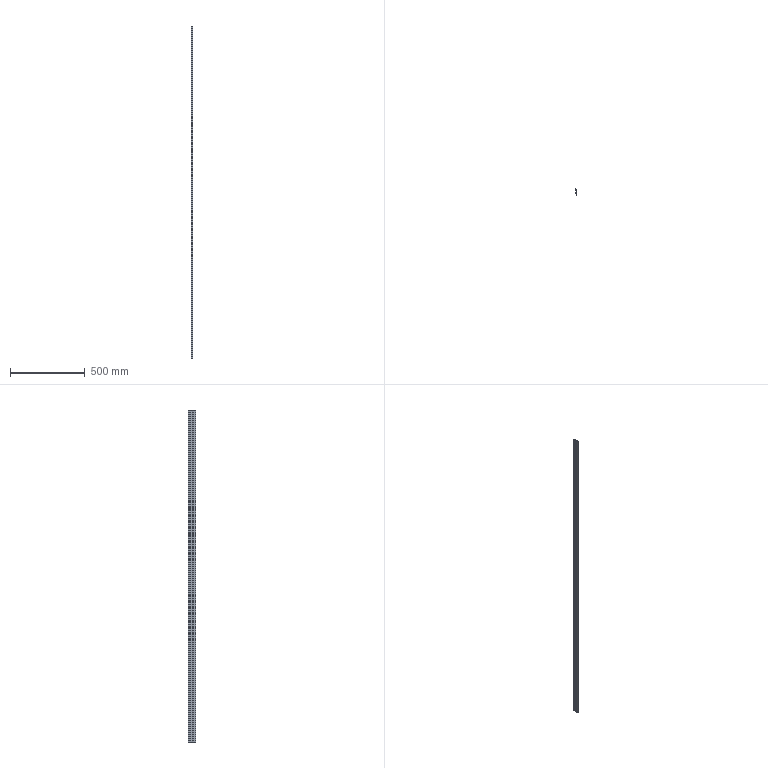Part | SolidWorks | features Extrusion 1 | 1 solid | 33 faces | box 9.4 x 46.998 x 2216 mm | volume 250321 mm3 | plane 22 | cylinder 11 | commonest cylinder face diameters 0.24 x2 0.4 x2 0.8 x2 1.2 x2 6 x2 1 x1
STEP:
#1=CARTESIAN_POINT('',(-2.9,32.45,-1108.));
#2=VERTEX_POINT('',#1);
#3=CARTESIAN_POINT('',(-2.7,32.25,-1108.));
#4=VERTEX_POINT('',#3);
#5=CARTESIAN_POINT('',(-2.7,32.45,-1108.));
#6=DIRECTION('',(0.,0.,1.));
#7=DIRECTION('',(1.,0.,0.));
#8=AXIS2_PLACEMENT_3D('',#5,#6,#7);
#9=CIRCLE('',#8,0.2);
#10=EDGE_CURVE('',#2,#4,#9,.T.);
#11=ORIENTED_EDGE('',*,*,#10,.T.);
#12=CARTESIAN_POINT('',(-2.7,32.25,1108.));
#13=VERTEX_POINT('',#12);
#14=CARTESIAN_POINT('',(-2.7,32.25,1108.));
#15=DIRECTION('',(0.,0.,-1.));
#16=VECTOR('',#15,1000.);
#17=LINE('',#14,#16);
#18=EDGE_CURVE('',#13,#4,#17,.T.);
#19=ORIENTED_EDGE('',*,*,#18,.F.);
#20=CARTESIAN_POINT('',(-2.9,32.45,1108.));
#21=VERTEX_POINT('',#20);
#22=CARTESIAN_POINT('',(-2.7,32.45,1108.));
#23=DIRECTION('',(0.,0.,1.));
#24=DIRECTION('',(1.,0.,0.));
#25=AXIS2_PLACEMENT_3D('',#22,#23,#24);
#26=CIRCLE('',#25,0.2);
#27=EDGE_CURVE('',#21,#13,#26,.T.);
#28=ORIENTED_EDGE('',*,*,#27,.F.);
#29=CARTESIAN_POINT('',(-2.9,32.45,1108.));
#30=DIRECTION('',(0.,0.,-1.));
#31=VECTOR('',#30,1000.);
#32=LINE('',#29,#31);
#33=EDGE_CURVE('',#21,#2,#32,.T.);
#34=ORIENTED_EDGE('',*,*,#33,.T.);
#35=EDGE_LOOP('',(#11,#19,#28,#34));
#36=FACE_OUTER_BOUND('',#35,.T.);
#37=CARTESIAN_POINT('',(-2.7,32.45,1108.));
#38=DIRECTION('',(0.,0.,-1.));
#39=DIRECTION('',(-1.,0.,0.));
#40=AXIS2_PLACEMENT_3D('',#37,#38,#39);
#41=CYLINDRICAL_SURFACE('',#40,0.2);
#42=ADVANCED_FACE('',(#36),#41,.T.);
#43=CARTESIAN_POINT('',(-2.5,32.25,-1108.));
#44=VERTEX_POINT('',#43);
#45=CARTESIAN_POINT('',(-2.7,32.25,-1108.));
#46=DIRECTION('',(1.,0.,0.));
#47=VECTOR('',#46,1000.);
#48=LINE('',#45,#47);
#49=EDGE_CURVE('',#4,#44,#48,.T.);
#50=ORIENTED_EDGE('',*,*,#49,.T.);
#51=CARTESIAN_POINT('',(-2.5,32.25,1108.));
#52=VERTEX_POINT('',#51);
#53=CARTESIAN_POINT('',(-2.5,32.25,1108.));
#54=DIRECTION('',(0.,0.,-1.));
#55=VECTOR('',#54,1000.);
#56=LINE('',#53,#55);
#57=EDGE_CURVE('',#52,#44,#56,.T.);
#58=ORIENTED_EDGE('',*,*,#57,.F.);
#59=CARTESIAN_POINT('',(-2.7,32.25,1108.));
#60=DIRECTION('',(1.,0.,0.));
#61=VECTOR('',#60,1000.);
#62=LINE('',#59,#61);
#63=EDGE_CURVE('',#13,#52,#62,.T.);
#64=ORIENTED_EDGE('',*,*,#63,.F.);
#65=ORIENTED_EDGE('',*,*,#18,.T.);
#66=EDGE_LOOP('',(#50,#58,#64,#65));
#67=FACE_OUTER_BOUND('',#66,.T.);
#68=CARTESIAN_POINT('',(-2.7,32.25,1108.));
#69=DIRECTION('',(0.,1.,0.));
#70=DIRECTION('',(0.,0.,1.));
#71=AXIS2_PLACEMENT_3D('',#68,#69,#70);
#72=PLANE('',#71);
#73=ADVANCED_FACE('',(#67),#72,.F.);
#74=CARTESIAN_POINT('',(-1.9,32.85,-1108.));
#75=VERTEX_POINT('',#74);
#76=CARTESIAN_POINT('',(-2.5,32.85,-1108.));
#77=DIRECTION('',(0.,0.,1.));
#78=DIRECTION('',(1.,0.,0.));
#79=AXIS2_PLACEMENT_3D('',#76,#77,#78);
#80=CIRCLE('',#79,0.6);
#81=EDGE_CURVE('',#44,#75,#80,.T.);
#82=ORIENTED_EDGE('',*,*,#81,.T.);
#83=CARTESIAN_POINT('',(-1.9,32.85,1108.));
#84=VERTEX_POINT('',#83);
#85=CARTESIAN_POINT('',(-1.9,32.85,1108.));
#86=DIRECTION('',(0.,0.,-1.));
#87=VECTOR('',#86,1000.);
#88=LINE('',#85,#87);
#89=EDGE_CURVE('',#84,#75,#88,.T.);
#90=ORIENTED_EDGE('',*,*,#89,.F.);
#91=CARTESIAN_POINT('',(-2.5,32.85,1108.));
#92=DIRECTION('',(0.,0.,1.));
#93=DIRECTION('',(1.,0.,0.));
#94=AXIS2_PLACEMENT_3D('',#91,#92,#93);
#95=CIRCLE('',#94,0.6);
#96=EDGE_CURVE('',#52,#84,#95,.T.);
#97=ORIENTED_EDGE('',*,*,#96,.F.);
#98=ORIENTED_EDGE('',*,*,#57,.T.);
#99=EDGE_LOOP('',(#82,#90,#97,#98));
#100=FACE_OUTER_BOUND('',#99,.T.);
#101=CARTESIAN_POINT('',(-2.5,32.85,1108.));
#102=DIRECTION('',(0.,0.,-1.));
#103=DIRECTION('',(-1.,0.,0.));
#104=AXIS2_PLACEMENT_3D('',#101,#102,#103);
#105=CYLINDRICAL_SURFACE('',#104,0.6);
#106=ADVANCED_FACE('',(#100),#105,.T.);
#107=CARTESIAN_POINT('',(-1.9,36.13,-1108.));
#108=VERTEX_POINT('',#107);
#109=CARTESIAN_POINT('',(-1.9,32.85,-1108.));
#110=DIRECTION('',(0.,1.,0.));
#111=VECTOR('',#110,1000.);
#112=LINE('',#109,#111);
#113=EDGE_CURVE('',#75,#108,#112,.T.);
#114=ORIENTED_EDGE('',*,*,#113,.T.);
#115=CARTESIAN_POINT('',(-1.9,36.13,1108.));
#116=VERTEX_POINT('',#115);
#117=CARTESIAN_POINT('',(-1.9,36.13,1108.));
#118=DIRECTION('',(0.,0.,-1.));
#119=VECTOR('',#118,1000.);
#120=LINE('',#117,#119);
#121=EDGE_CURVE('',#116,#108,#120,.T.);
#122=ORIENTED_EDGE('',*,*,#121,.F.);
#123=CARTESIAN_POINT('',(-1.9,32.85,1108.));
#124=DIRECTION('',(0.,1.,0.));
#125=VECTOR('',#124,1000.);
#126=LINE('',#123,#125);
#127=EDGE_CURVE('',#84,#116,#126,.T.);
#128=ORIENTED_EDGE('',*,*,#127,.F.);
#129=ORIENTED_EDGE('',*,*,#89,.T.);
#130=EDGE_LOOP('',(#114,#122,#128,#129));
#131=FACE_OUTER_BOUND('',#130,.T.);
#132=CARTESIAN_POINT('',(-1.9,32.85,1108.));
#133=DIRECTION('',(-1.,0.,0.));
#134=DIRECTION('',(0.,0.,1.));
#135=AXIS2_PLACEMENT_3D('',#132,#133,#134);
#136=PLANE('',#135);
#137=ADVANCED_FACE('',(#131),#136,.F.);
#138=CARTESIAN_POINT('',(-1.78,36.25,-1108.));
#139=VERTEX_POINT('',#138);
#140=CARTESIAN_POINT('',(-1.78,36.13,-1108.));
#141=DIRECTION('',(0.,0.,-1.));
#142=DIRECTION('',(1.,0.,0.));
#143=AXIS2_PLACEMENT_3D('',#140,#141,#142);
#144=CIRCLE('',#143,0.12);
#145=EDGE_CURVE('',#108,#139,#144,.T.);
#146=ORIENTED_EDGE('',*,*,#145,.T.);
#147=CARTESIAN_POINT('',(-1.78,36.25,1108.));
#148=VERTEX_POINT('',#147);
#149=CARTESIAN_POINT('',(-1.78,36.25,1108.));
#150=DIRECTION('',(0.,0.,-1.));
#151=VECTOR('',#150,1000.);
#152=LINE('',#149,#151);
#153=EDGE_CURVE('',#148,#139,#152,.T.);
#154=ORIENTED_EDGE('',*,*,#153,.F.);
#155=CARTESIAN_POINT('',(-1.78,36.13,1108.));
#156=DIRECTION('',(0.,0.,-1.));
#157=DIRECTION('',(1.,0.,0.));
#158=AXIS2_PLACEMENT_3D('',#155,#156,#157);
#159=CIRCLE('',#158,0.12);
#160=EDGE_CURVE('',#116,#148,#159,.T.);
#161=ORIENTED_EDGE('',*,*,#160,.F.);
#162=ORIENTED_EDGE('',*,*,#121,.T.);
#163=EDGE_LOOP('',(#146,#154,#161,#162));
#164=FACE_OUTER_BOUND('',#163,.T.);
#165=CARTESIAN_POINT('',(-1.78,36.13,1108.));
#166=DIRECTION('',(0.,0.,-1.));
#167=DIRECTION('',(-1.,0.,0.));
#168=AXIS2_PLACEMENT_3D('',#165,#166,#167);
#169=CYLINDRICAL_SURFACE('',#168,0.12);
#170=ADVANCED_FACE('',(#164),#169,.F.);
#171=CARTESIAN_POINT('',(0.,36.25,-1108.));
#172=VERTEX_POINT('',#171);
#173=CARTESIAN_POINT('',(-1.78,36.25,-1108.));
#174=DIRECTION('',(1.,0.,0.));
#175=VECTOR('',#174,1000.);
#176=LINE('',#173,#175);
#177=EDGE_CURVE('',#139,#172,#176,.T.);
#178=ORIENTED_EDGE('',*,*,#177,.T.);
#179=CARTESIAN_POINT('',(0.,36.25,1108.));
#180=VERTEX_POINT('',#179);
#181=CARTESIAN_POINT('',(0.,36.25,1108.));
#182=DIRECTION('',(0.,0.,-1.));
#183=VECTOR('',#182,1000.);
#184=LINE('',#181,#183);
#185=EDGE_CURVE('',#180,#172,#184,.T.);
#186=ORIENTED_EDGE('',*,*,#185,.F.);
#187=CARTESIAN_POINT('',(-1.78,36.25,1108.));
#188=DIRECTION('',(1.,0.,0.));
#189=VECTOR('',#188,1000.);
#190=LINE('',#187,#189);
#191=EDGE_CURVE('',#148,#180,#190,.T.);
#192=ORIENTED_EDGE('',*,*,#191,.F.);
#193=ORIENTED_EDGE('',*,*,#153,.T.);
#194=EDGE_LOOP('',(#178,#186,#192,#193));
#195=FACE_OUTER_BOUND('',#194,.T.);
#196=CARTESIAN_POINT('',(-1.78,36.25,1108.));
#197=DIRECTION('',(0.,1.,0.));
#198=DIRECTION('',(0.,0.,1.));
#199=AXIS2_PLACEMENT_3D('',#196,#197,#198);
#200=PLANE('',#199);
#201=ADVANCED_FACE('',(#195),#200,.F.);
#202=CARTESIAN_POINT('',(0.0007641,20.449,-1108.));
#203=VERTEX_POINT('',#202);
#204=CARTESIAN_POINT('',(0.,36.25,-1108.));
#205=DIRECTION('',(0.00004836,-1.,0.));
#206=VECTOR('',#205,1000.);
#207=LINE('',#204,#206);
#208=EDGE_CURVE('',#172,#203,#207,.T.);
#209=ORIENTED_EDGE('',*,*,#208,.T.);
#210=CARTESIAN_POINT('',(0.0007641,20.449,1108.));
#211=VERTEX_POINT('',#210);
#212=CARTESIAN_POINT('',(0.0007641,20.449,1108.));
#213=DIRECTION('',(0.,0.,-1.));
#214=VECTOR('',#213,1000.);
#215=LINE('',#212,#214);
#216=EDGE_CURVE('',#211,#203,#215,.T.);
#217=ORIENTED_EDGE('',*,*,#216,.F.);
#218=CARTESIAN_POINT('',(0.,36.25,1108.));
#219=DIRECTION('',(0.00004836,-1.,0.));
#220=VECTOR('',#219,1000.);
#221=LINE('',#218,#220);
#222=EDGE_CURVE('',#180,#211,#221,.T.);
#223=ORIENTED_EDGE('',*,*,#222,.F.);
#224=ORIENTED_EDGE('',*,*,#185,.T.);
#225=EDGE_LOOP('',(#209,#217,#223,#224));
#226=FACE_OUTER_BOUND('',#225,.T.);
#227=CARTESIAN_POINT('',(0.,36.25,1108.));
#228=DIRECTION('',(1.,0.00004836,0.));
#229=DIRECTION('',(-0.00004836,1.,0.));
#230=AXIS2_PLACEMENT_3D('',#227,#228,#229);
#231=PLANE('',#230);
#232=ADVANCED_FACE('',(#226),#231,.F.);
#233=CARTESIAN_POINT('',(-2.499,20.449,-1108.));
#234=VERTEX_POINT('',#233);
#235=CARTESIAN_POINT('',(0.0007641,20.449,-1108.));
#236=DIRECTION('',(-1.,0.,0.));
#237=VECTOR('',#236,1000.);
#238=LINE('',#235,#237);
#239=EDGE_CURVE('',#203,#234,#238,.T.);
#240=ORIENTED_EDGE('',*,*,#239,.T.);
#241=CARTESIAN_POINT('',(-2.499,20.449,1108.));
#242=VERTEX_POINT('',#241);
#243=CARTESIAN_POINT('',(-2.499,20.449,1108.));
#244=DIRECTION('',(0.,0.,-1.));
#245=VECTOR('',#244,1000.);
#246=LINE('',#243,#245);
#247=EDGE_CURVE('',#242,#234,#246,.T.);
#248=ORIENTED_EDGE('',*,*,#247,.F.);
#249=CARTESIAN_POINT('',(0.0007641,20.449,1108.));
#250=DIRECTION('',(-1.,0.,0.));
#251=VECTOR('',#250,1000.);
#252=LINE('',#249,#251);
#253=EDGE_CURVE('',#211,#242,#252,.T.);
#254=ORIENTED_EDGE('',*,*,#253,.F.);
#255=ORIENTED_EDGE('',*,*,#216,.T.);
#256=EDGE_LOOP('',(#240,#248,#254,#255));
#257=FACE_OUTER_BOUND('',#256,.T.);
#258=CARTESIAN_POINT('',(0.0007641,20.449,1108.));
#259=DIRECTION('',(0.,-1.,0.));
#260=DIRECTION('',(0.,0.,-1.));
#261=AXIS2_PLACEMENT_3D('',#258,#259,#260);
#262=PLANE('',#261);
#263=ADVANCED_FACE('',(#257),#262,.F.);
#264=CARTESIAN_POINT('',(-2.899,20.049,-1108.));
#265=VERTEX_POINT('',#264);
#266=CARTESIAN_POINT('',(-2.499,20.049,-1108.));
#267=DIRECTION('',(0.,0.,1.));
#268=DIRECTION('',(1.,0.,0.));
#269=AXIS2_PLACEMENT_3D('',#266,#267,#268);
#270=CIRCLE('',#269,0.4);
#271=EDGE_CURVE('',#234,#265,#270,.T.);
#272=ORIENTED_EDGE('',*,*,#271,.T.);
#273=CARTESIAN_POINT('',(-2.899,20.049,1108.));
#274=VERTEX_POINT('',#273);
#275=CARTESIAN_POINT('',(-2.899,20.049,1108.));
#276=DIRECTION('',(0.,0.,-1.));
#277=VECTOR('',#276,1000.);
#278=LINE('',#275,#277);
#279=EDGE_CURVE('',#274,#265,#278,.T.);
#280=ORIENTED_EDGE('',*,*,#279,.F.);
#281=CARTESIAN_POINT('',(-2.499,20.049,1108.));
#282=DIRECTION('',(0.,0.,1.));
#283=DIRECTION('',(1.,0.,0.));
#284=AXIS2_PLACEMENT_3D('',#281,#282,#283);
#285=CIRCLE('',#284,0.4);
#286=EDGE_CURVE('',#242,#274,#285,.T.);
#287=ORIENTED_EDGE('',*,*,#286,.F.);
#288=ORIENTED_EDGE('',*,*,#247,.T.);
#289=EDGE_LOOP('',(#272,#280,#287,#288));
#290=FACE_OUTER_BOUND('',#289,.T.);
#291=CARTESIAN_POINT('',(-2.499,20.049,1108.));
#292=DIRECTION('',(0.,0.,-1.));
#293=DIRECTION('',(-1.,0.,0.));
#294=AXIS2_PLACEMENT_3D('',#291,#292,#293);
#295=CYLINDRICAL_SURFACE('',#294,0.4);
#296=ADVANCED_FACE('',(#290),#295,.T.);
#297=CARTESIAN_POINT('',(-2.899,15.65,-1108.));
#298=VERTEX_POINT('',#297);
#299=CARTESIAN_POINT('',(-2.899,20.049,-1108.));
#300=DIRECTION('',(0.,-1.,0.));
#301=VECTOR('',#300,1000.);
#302=LINE('',#299,#301);
#303=EDGE_CURVE('',#265,#298,#302,.T.);
#304=ORIENTED_EDGE('',*,*,#303,.T.);
#305=CARTESIAN_POINT('',(-2.899,15.65,1108.));
#306=VERTEX_POINT('',#305);
#307=CARTESIAN_POINT('',(-2.899,15.65,1108.));
#308=DIRECTION('',(0.,0.,-1.));
#309=VECTOR('',#308,1000.);
#310=LINE('',#307,#309);
#311=EDGE_CURVE('',#306,#298,#310,.T.);
#312=ORIENTED_EDGE('',*,*,#311,.F.);
#313=CARTESIAN_POINT('',(-2.899,20.049,1108.));
#314=DIRECTION('',(0.,-1.,0.));
#315=VECTOR('',#314,1000.);
#316=LINE('',#313,#315);
#317=EDGE_CURVE('',#274,#306,#316,.T.);
#318=ORIENTED_EDGE('',*,*,#317,.F.);
#319=ORIENTED_EDGE('',*,*,#279,.T.);
#320=EDGE_LOOP('',(#304,#312,#318,#319));
#321=FACE_OUTER_BOUND('',#320,.T.);
#322=CARTESIAN_POINT('',(-2.899,20.049,1108.));
#323=DIRECTION('',(1.,0.,0.));
#324=DIRECTION('',(0.,0.,-1.));
#325=AXIS2_PLACEMENT_3D('',#322,#323,#324);
#326=PLANE('',#325);
#327=ADVANCED_FACE('',(#321),#326,.F.);
#328=CARTESIAN_POINT('',(-2.699,15.45,-1108.));
#329=VERTEX_POINT('',#328);
#330=CARTESIAN_POINT('',(-2.699,15.65,-1108.));
#331=DIRECTION('',(0.,0.,1.));
#332=DIRECTION('',(1.,0.,0.));
#333=AXIS2_PLACEMENT_3D('',#330,#331,#332);
#334=CIRCLE('',#333,0.2);
#335=EDGE_CURVE('',#298,#329,#334,.T.);
#336=ORIENTED_EDGE('',*,*,#335,.T.);
#337=CARTESIAN_POINT('',(-2.699,15.45,1108.));
#338=VERTEX_POINT('',#337);
#339=CARTESIAN_POINT('',(-2.699,15.45,1108.));
#340=DIRECTION('',(0.,0.,-1.));
#341=VECTOR('',#340,1000.);
#342=LINE('',#339,#341);
#343=EDGE_CURVE('',#338,#329,#342,.T.);
#344=ORIENTED_EDGE('',*,*,#343,.F.);
#345=CARTESIAN_POINT('',(-2.699,15.65,1108.));
#346=DIRECTION('',(0.,0.,1.));
#347=DIRECTION('',(1.,0.,0.));
#348=AXIS2_PLACEMENT_3D('',#345,#346,#347);
#349=CIRCLE('',#348,0.2);
#350=EDGE_CURVE('',#306,#338,#349,.T.);
#351=ORIENTED_EDGE('',*,*,#350,.F.);
#352=ORIENTED_EDGE('',*,*,#311,.T.);
#353=EDGE_LOOP('',(#336,#344,#351,#352));
#354=FACE_OUTER_BOUND('',#353,.T.);
#355=CARTESIAN_POINT('',(-2.699,15.65,1108.));
#356=DIRECTION('',(0.,0.,-1.));
#357=DIRECTION('',(-1.,0.,0.));
#358=AXIS2_PLACEMENT_3D('',#355,#356,#357);
#359=CYLINDRICAL_SURFACE('',#358,0.2);
#360=ADVANCED_FACE('',(#354),#359,.T.);
#361=CARTESIAN_POINT('',(-2.499,15.45,-1108.));
#362=VERTEX_POINT('',#361);
#363=CARTESIAN_POINT('',(-2.699,15.45,-1108.));
#364=DIRECTION('',(1.,0.,0.));
#365=VECTOR('',#364,1000.);
#366=LINE('',#363,#365);
#367=EDGE_CURVE('',#329,#362,#366,.T.);
#368=ORIENTED_EDGE('',*,*,#367,.T.);
#369=CARTESIAN_POINT('',(-2.499,15.45,1108.));
#370=VERTEX_POINT('',#369);
#371=CARTESIAN_POINT('',(-2.499,15.45,1108.));
#372=DIRECTION('',(0.,0.,-1.));
#373=VECTOR('',#372,1000.);
#374=LINE('',#371,#373);
#375=EDGE_CURVE('',#370,#362,#374,.T.);
#376=ORIENTED_EDGE('',*,*,#375,.F.);
#377=CARTESIAN_POINT('',(-2.699,15.45,1108.));
#378=DIRECTION('',(1.,0.,0.));
#379=VECTOR('',#378,1000.);
#380=LINE('',#377,#379);
#381=EDGE_CURVE('',#338,#370,#380,.T.);
#382=ORIENTED_EDGE('',*,*,#381,.F.);
#383=ORIENTED_EDGE('',*,*,#343,.T.);
#384=EDGE_LOOP('',(#368,#376,#382,#383));
#385=FACE_OUTER_BOUND('',#384,.T.);
#386=CARTESIAN_POINT('',(-2.699,15.45,1108.));
#387=DIRECTION('',(0.,1.,0.));
#388=DIRECTION('',(0.,0.,1.));
#389=AXIS2_PLACEMENT_3D('',#386,#387,#388);
#390=PLANE('',#389);
#391=ADVANCED_FACE('',(#385),#390,.F.);
#392=CARTESIAN_POINT('',(-1.899,16.05,-1108.));
#393=VERTEX_POINT('',#392);
#394=CARTESIAN_POINT('',(-2.499,16.05,-1108.));
#395=DIRECTION('',(0.,0.,1.));
#396=DIRECTION('',(1.,0.,0.));
#397=AXIS2_PLACEMENT_3D('',#394,#395,#396);
#398=CIRCLE('',#397,0.6);
#399=EDGE_CURVE('',#362,#393,#398,.T.);
#400=ORIENTED_EDGE('',*,*,#399,.T.);
#401=CARTESIAN_POINT('',(-1.899,16.05,1108.));
#402=VERTEX_POINT('',#401);
#403=CARTESIAN_POINT('',(-1.899,16.05,1108.));
#404=DIRECTION('',(0.,0.,-1.));
#405=VECTOR('',#404,1000.);
#406=LINE('',#403,#405);
#407=EDGE_CURVE('',#402,#393,#406,.T.);
#408=ORIENTED_EDGE('',*,*,#407,.F.);
#409=CARTESIAN_POINT('',(-2.499,16.05,1108.));
#410=DIRECTION('',(0.,0.,1.));
#411=DIRECTION('',(1.,0.,0.));
#412=AXIS2_PLACEMENT_3D('',#409,#410,#411);
#413=CIRCLE('',#412,0.6);
#414=EDGE_CURVE('',#370,#402,#413,.T.);
#415=ORIENTED_EDGE('',*,*,#414,.F.);
#416=ORIENTED_EDGE('',*,*,#375,.T.);
#417=EDGE_LOOP('',(#400,#408,#415,#416));
#418=FACE_OUTER_BOUND('',#417,.T.);
#419=CARTESIAN_POINT('',(-2.499,16.05,1108.));
#420=DIRECTION('',(0.,0.,-1.));
#421=DIRECTION('',(-1.,0.,0.));
#422=AXIS2_PLACEMENT_3D('',#419,#420,#421);
#423=CYLINDRICAL_SURFACE('',#422,0.6);
#424=ADVANCED_FACE('',(#418),#423,.T.);
#425=CARTESIAN_POINT('',(-1.899,19.329,-1108.));
#426=VERTEX_POINT('',#425);
#427=CARTESIAN_POINT('',(-1.899,16.05,-1108.));
#428=DIRECTION('',(0.,1.,0.));
#429=VECTOR('',#428,1000.);
#430=LINE('',#427,#429);
#431=EDGE_CURVE('',#393,#426,#430,.T.);
#432=ORIENTED_EDGE('',*,*,#431,.T.);
#433=CARTESIAN_POINT('',(-1.899,19.329,1108.));
#434=VERTEX_POINT('',#433);
#435=CARTESIAN_POINT('',(-1.899,19.329,1108.));
#436=DIRECTION('',(0.,0.,-1.));
#437=VECTOR('',#436,1000.);
#438=LINE('',#435,#437);
#439=EDGE_CURVE('',#434,#426,#438,.T.);
#440=ORIENTED_EDGE('',*,*,#439,.F.);
#441=CARTESIAN_POINT('',(-1.899,16.05,1108.));
#442=DIRECTION('',(0.,1.,0.));
#443=VECTOR('',#442,1000.);
#444=LINE('',#441,#443);
#445=EDGE_CURVE('',#402,#434,#444,.T.);
#446=ORIENTED_EDGE('',*,*,#445,.F.);
#447=ORIENTED_EDGE('',*,*,#407,.T.);
#448=EDGE_LOOP('',(#432,#440,#446,#447));
#449=FACE_OUTER_BOUND('',#448,.T.);
#450=CARTESIAN_POINT('',(-1.899,16.05,1108.));
#451=DIRECTION('',(-1.,0.,0.));
#452=DIRECTION('',(0.,0.,1.));
#453=AXIS2_PLACEMENT_3D('',#450,#451,#452);
#454=PLANE('',#453);
#455=ADVANCED_FACE('',(#449),#454,.F.);
#456=CARTESIAN_POINT('',(-1.779,19.449,-1108.));
#457=VERTEX_POINT('',#456);
#458=CARTESIAN_POINT('',(-1.779,19.329,-1108.));
#459=DIRECTION('',(0.,0.,-1.));
#460=DIRECTION('',(1.,0.,0.));
#461=AXIS2_PLACEMENT_3D('',#458,#459,#460);
#462=CIRCLE('',#461,0.12);
#463=EDGE_CURVE('',#426,#457,#462,.T.);
#464=ORIENTED_EDGE('',*,*,#463,.T.);
#465=CARTESIAN_POINT('',(-1.779,19.449,1108.));
#466=VERTEX_POINT('',#465);
#467=CARTESIAN_POINT('',(-1.779,19.449,1108.));
#468=DIRECTION('',(0.,0.,-1.));
#469=VECTOR('',#468,1000.);
#470=LINE('',#467,#469);
#471=EDGE_CURVE('',#466,#457,#470,.T.);
#472=ORIENTED_EDGE('',*,*,#471,.F.);
#473=CARTESIAN_POINT('',(-1.779,19.329,1108.));
#474=DIRECTION('',(0.,0.,-1.));
#475=DIRECTION('',(1.,0.,0.));
#476=AXIS2_PLACEMENT_3D('',#473,#474,#475);
#477=CIRCLE('',#476,0.12);
#478=EDGE_CURVE('',#434,#466,#477,.T.);
#479=ORIENTED_EDGE('',*,*,#478,.F.);
#480=ORIENTED_EDGE('',*,*,#439,.T.);
#481=EDGE_LOOP('',(#464,#472,#479,#480));
#482=FACE_OUTER_BOUND('',#481,.T.);
#483=CARTESIAN_POINT('',(-1.779,19.329,1108.));
#484=DIRECTION('',(0.,0.,-1.));
#485=DIRECTION('',(-1.,0.,0.));
#486=AXIS2_PLACEMENT_3D('',#483,#484,#485);
#487=CYLINDRICAL_SURFACE('',#486,0.12);
#488=ADVANCED_FACE('',(#482),#487,.F.);
#489=CARTESIAN_POINT('',(0.0007641,19.449,-1108.));
#490=VERTEX_POINT('',#489);
#491=CARTESIAN_POINT('',(-1.779,19.449,-1108.));
#492=DIRECTION('',(1.,0.,0.));
#493=VECTOR('',#492,1000.);
#494=LINE('',#491,#493);
#495=EDGE_CURVE('',#457,#490,#494,.T.);
#496=ORIENTED_EDGE('',*,*,#495,.T.);
#497=CARTESIAN_POINT('',(0.0007641,19.449,1108.));
#498=VERTEX_POINT('',#497);
#499=CARTESIAN_POINT('',(0.0007641,19.449,1108.));
#500=DIRECTION('',(0.,0.,-1.));
#501=VECTOR('',#500,1000.);
#502=LINE('',#499,#501);
#503=EDGE_CURVE('',#498,#490,#502,.T.);
#504=ORIENTED_EDGE('',*,*,#503,.F.);
#505=CARTESIAN_POINT('',(-1.779,19.449,1108.));
#506=DIRECTION('',(1.,0.,0.));
#507=VECTOR('',#506,1000.);
#508=LINE('',#505,#507);
#509=EDGE_CURVE('',#466,#498,#508,.T.);
#510=ORIENTED_EDGE('',*,*,#509,.F.);
#511=ORIENTED_EDGE('',*,*,#471,.T.);
#512=EDGE_LOOP('',(#496,#504,#510,#511));
#513=FACE_OUTER_BOUND('',#512,.T.);
#514=CARTESIAN_POINT('',(-1.779,19.449,1108.));
#515=DIRECTION('',(0.,1.,0.));
#516=DIRECTION('',(0.,0.,1.));
#517=AXIS2_PLACEMENT_3D('',#514,#515,#516);
#518=PLANE('',#517);
#519=ADVANCED_FACE('',(#513),#518,.F.);
#520=CARTESIAN_POINT('',(0.,0.,-1108.));
#521=VERTEX_POINT('',#520);
#522=CARTESIAN_POINT('',(0.0007641,19.449,-1108.));
#523=DIRECTION('',(-0.00003929,-1.,0.));
#524=VECTOR('',#523,1000.);
#525=LINE('',#522,#524);
#526=EDGE_CURVE('',#490,#521,#525,.T.);
#527=ORIENTED_EDGE('',*,*,#526,.T.);
#528=CARTESIAN_POINT('',(0.,0.,1108.));
#529=VERTEX_POINT('',#528);
#530=CARTESIAN_POINT('',(0.,0.,1108.));
#531=DIRECTION('',(0.,0.,-1.));
#532=VECTOR('',#531,1000.);
#533=LINE('',#530,#532);
#534=EDGE_CURVE('',#529,#521,#533,.T.);
#535=ORIENTED_EDGE('',*,*,#534,.F.);
#536=CARTESIAN_POINT('',(0.0007641,19.449,1108.));
#537=DIRECTION('',(-0.00003929,-1.,0.));
#538=VECTOR('',#537,1000.);
#539=LINE('',#536,#538);
#540=EDGE_CURVE('',#498,#529,#539,.T.);
#541=ORIENTED_EDGE('',*,*,#540,.F.);
#542=ORIENTED_EDGE('',*,*,#503,.T.);
#543=EDGE_LOOP('',(#527,#535,#541,#542));
#544=FACE_OUTER_BOUND('',#543,.T.);
#545=CARTESIAN_POINT('',(0.0007641,19.449,1108.));
#546=DIRECTION('',(1.,-0.00003929,0.));
#547=DIRECTION('',(0.00003929,1.,0.));
#548=AXIS2_PLACEMENT_3D('',#545,#546,#547);
#549=PLANE('',#548);
#550=ADVANCED_FACE('',(#544),#549,.F.);
#551=CARTESIAN_POINT('',(1.5,0.,-1108.));
#552=VERTEX_POINT('',#551);
#553=CARTESIAN_POINT('',(0.,0.,-1108.));
#554=DIRECTION('',(1.,0.,0.));
#555=VECTOR('',#554,1000.);
#556=LINE('',#553,#555);
#557=EDGE_CURVE('',#521,#552,#556,.T.);
#558=ORIENTED_EDGE('',*,*,#557,.T.);
#559=CARTESIAN_POINT('',(1.5,0.,1108.));
#560=VERTEX_POINT('',#559);
#561=CARTESIAN_POINT('',(1.5,0.,1108.));
#562=DIRECTION('',(0.,0.,-1.));
#563=VECTOR('',#562,1000.);
#564=LINE('',#561,#563);
#565=EDGE_CURVE('',#560,#552,#564,.T.);
#566=ORIENTED_EDGE('',*,*,#565,.F.);
#567=CARTESIAN_POINT('',(0.,0.,1108.));
#568=DIRECTION('',(1.,0.,0.));
#569=VECTOR('',#568,1000.);
#570=LINE('',#567,#569);
#571=EDGE_CURVE('',#529,#560,#570,.T.);
#572=ORIENTED_EDGE('',*,*,#571,.F.);
#573=ORIENTED_EDGE('',*,*,#534,.T.);
#574=EDGE_LOOP('',(#558,#566,#572,#573));
#575=FACE_OUTER_BOUND('',#574,.T.);
#576=CARTESIAN_POINT('',(0.,0.,1108.));
#577=DIRECTION('',(0.,1.,0.));
#578=DIRECTION('',(0.,0.,1.));
#579=AXIS2_PLACEMENT_3D('',#576,#577,#578);
#580=PLANE('',#579);
#581=ADVANCED_FACE('',(#575),#580,.F.);
#582=CARTESIAN_POINT('',(2.,0.5,-1108.));
#583=VERTEX_POINT('',#582);
#584=CARTESIAN_POINT('',(1.5,0.5,-1108.));
#585=DIRECTION('',(0.,0.,1.));
#586=DIRECTION('',(1.,0.,0.));
#587=AXIS2_PLACEMENT_3D('',#584,#585,#586);
#588=CIRCLE('',#587,0.5);
#589=EDGE_CURVE('',#552,#583,#588,.T.);
#590=ORIENTED_EDGE('',*,*,#589,.T.);
#591=CARTESIAN_POINT('',(2.,0.5,1108.));
#592=VERTEX_POINT('',#591);
#593=CARTESIAN_POINT('',(2.,0.5,1108.));
#594=DIRECTION('',(0.,0.,-1.));
#595=VECTOR('',#594,1000.);
#596=LINE('',#593,#595);
#597=EDGE_CURVE('',#592,#583,#596,.T.);
#598=ORIENTED_EDGE('',*,*,#597,.F.);
#599=CARTESIAN_POINT('',(1.5,0.5,1108.));
#600=DIRECTION('',(0.,0.,1.));
#601=DIRECTION('',(1.,0.,0.));
#602=AXIS2_PLACEMENT_3D('',#599,#600,#601);
#603=CIRCLE('',#602,0.5);
#604=EDGE_CURVE('',#560,#592,#603,.T.);
#605=ORIENTED_EDGE('',*,*,#604,.F.);
#606=ORIENTED_EDGE('',*,*,#565,.T.);
#607=EDGE_LOOP('',(#590,#598,#605,#606));
#608=FACE_OUTER_BOUND('',#607,.T.);
#609=CARTESIAN_POINT('',(1.5,0.5,1108.));
#610=DIRECTION('',(0.,0.,-1.));
#611=DIRECTION('',(-1.,0.,0.));
#612=AXIS2_PLACEMENT_3D('',#609,#610,#611);
#613=CYLINDRICAL_SURFACE('',#612,0.5);
#614=ADVANCED_FACE('',(#608),#613,.T.);
#615=CARTESIAN_POINT('',(2.,38.058,-1108.));
#616=VERTEX_POINT('',#615);
#617=CARTESIAN_POINT('',(2.,0.5,-1108.));
#618=DIRECTION('',(0.,1.,0.));
#619=VECTOR('',#618,1000.);
#620=LINE('',#617,#619);
#621=EDGE_CURVE('',#583,#616,#620,.T.);
#622=ORIENTED_EDGE('',*,*,#621,.T.);
#623=CARTESIAN_POINT('',(2.,38.058,1108.));
#624=VERTEX_POINT('',#623);
#625=CARTESIAN_POINT('',(2.,38.058,1108.));
#626=DIRECTION('',(0.,0.,-1.));
#627=VECTOR('',#626,1000.);
#628=LINE('',#625,#627);
#629=EDGE_CURVE('',#624,#616,#628,.T.);
#630=ORIENTED_EDGE('',*,*,#629,.F.);
#631=CARTESIAN_POINT('',(2.,0.5,1108.));
#632=DIRECTION('',(0.,1.,0.));
#633=VECTOR('',#632,1000.);
#634=LINE('',#631,#633);
#635=EDGE_CURVE('',#592,#624,#634,.T.);
#636=ORIENTED_EDGE('',*,*,#635,.F.);
#637=ORIENTED_EDGE('',*,*,#597,.T.);
#638=EDGE_LOOP('',(#622,#630,#636,#637));
#639=FACE_OUTER_BOUND('',#638,.T.);
#640=CARTESIAN_POINT('',(2.,0.5,1108.));
#641=DIRECTION('',(-1.,0.,0.));
#642=DIRECTION('',(0.,0.,1.));
#643=AXIS2_PLACEMENT_3D('',#640,#641,#642);
#644=PLANE('',#643);
#645=ADVANCED_FACE('',(#639),#644,.F.);
#646=CARTESIAN_POINT('',(1.393,39.868,-1108.));
#647=VERTEX_POINT('',#646);
#648=CARTESIAN_POINT('',(-1.,38.058,-1108.));
#649=DIRECTION('',(0.,0.,1.));
#650=DIRECTION('',(1.,0.,0.));
#651=AXIS2_PLACEMENT_3D('',#648,#649,#650);
#652=CIRCLE('',#651,3.);
#653=EDGE_CURVE('',#616,#647,#652,.T.);
#654=ORIENTED_EDGE('',*,*,#653,.T.);
#655=CARTESIAN_POINT('',(1.393,39.868,1108.));
#656=VERTEX_POINT('',#655);
#657=CARTESIAN_POINT('',(1.393,39.868,1108.));
#658=DIRECTION('',(0.,0.,-1.));
#659=VECTOR('',#658,1000.);
#660=LINE('',#657,#659);
#661=EDGE_CURVE('',#656,#647,#660,.T.);
#662=ORIENTED_EDGE('',*,*,#661,.F.);
#663=CARTESIAN_POINT('',(-1.,38.058,1108.));
#664=DIRECTION('',(0.,0.,1.));
#665=DIRECTION('',(1.,0.,0.));
#666=AXIS2_PLACEMENT_3D('',#663,#664,#665);
#667=CIRCLE('',#666,3.);
#668=EDGE_CURVE('',#624,#656,#667,.T.);
#669=ORIENTED_EDGE('',*,*,#668,.F.);
#670=ORIENTED_EDGE('',*,*,#629,.T.);
#671=EDGE_LOOP('',(#654,#662,#669,#670));
#672=FACE_OUTER_BOUND('',#671,.T.);
#673=CARTESIAN_POINT('',(-1.,38.058,1108.));
#674=DIRECTION('',(0.,0.,-1.));
#675=DIRECTION('',(-1.,0.,0.));
#676=AXIS2_PLACEMENT_3D('',#673,#674,#675);
#677=CYLINDRICAL_SURFACE('',#676,3.);
#678=ADVANCED_FACE('',(#672),#677,.T.);
#679=CARTESIAN_POINT('',(-4.,46.998,-1108.));
#680=VERTEX_POINT('',#679);
#681=CARTESIAN_POINT('',(1.393,39.868,-1108.));
#682=DIRECTION('',(-0.6032,0.7976,0.));
#683=VECTOR('',#682,1000.);
#684=LINE('',#681,#683);
#685=EDGE_CURVE('',#647,#680,#684,.T.);
#686=ORIENTED_EDGE('',*,*,#685,.T.);
#687=CARTESIAN_POINT('',(-4.,46.998,1108.));
#688=VERTEX_POINT('',#687);
#689=CARTESIAN_POINT('',(-4.,46.998,1108.));
#690=DIRECTION('',(0.,0.,-1.));
#691=VECTOR('',#690,1000.);
#692=LINE('',#689,#691);
#693=EDGE_CURVE('',#688,#680,#692,.T.);
#694=ORIENTED_EDGE('',*,*,#693,.F.);
#695=CARTESIAN_POINT('',(1.393,39.868,1108.));
#696=DIRECTION('',(-0.6032,0.7976,0.));
#697=VECTOR('',#696,1000.);
#698=LINE('',#695,#697);
#699=EDGE_CURVE('',#656,#688,#698,.T.);
#700=ORIENTED_EDGE('',*,*,#699,.F.);
#701=ORIENTED_EDGE('',*,*,#661,.T.);
#702=EDGE_LOOP('',(#686,#694,#700,#701));
#703=FACE_OUTER_BOUND('',#702,.T.);
#704=CARTESIAN_POINT('',(1.393,39.868,1108.));
#705=DIRECTION('',(-0.7976,-0.6032,0.));
#706=DIRECTION('',(0.6032,-0.7976,0.));
#707=AXIS2_PLACEMENT_3D('',#704,#705,#706);
#708=PLANE('',#707);
#709=ADVANCED_FACE('',(#703),#708,.F.);
#710=CARTESIAN_POINT('',(-7.4,46.998,-1108.));
#711=VERTEX_POINT('',#710);
#712=CARTESIAN_POINT('',(-4.,46.998,-1108.));
#713=DIRECTION('',(-1.,0.,0.));
#714=VECTOR('',#713,1000.);
#715=LINE('',#712,#714);
#716=EDGE_CURVE('',#680,#711,#715,.T.);
#717=ORIENTED_EDGE('',*,*,#716,.T.);
#718=CARTESIAN_POINT('',(-7.4,46.998,1108.));
#719=VERTEX_POINT('',#718);
#720=CARTESIAN_POINT('',(-7.4,46.998,1108.));
#721=DIRECTION('',(0.,0.,-1.));
#722=VECTOR('',#721,1000.);
#723=LINE('',#720,#722);
#724=EDGE_CURVE('',#719,#711,#723,.T.);
#725=ORIENTED_EDGE('',*,*,#724,.F.);
#726=CARTESIAN_POINT('',(-4.,46.998,1108.));
#727=DIRECTION('',(-1.,0.,0.));
#728=VECTOR('',#727,1000.);
#729=LINE('',#726,#728);
#730=EDGE_CURVE('',#688,#719,#729,.T.);
#731=ORIENTED_EDGE('',*,*,#730,.F.);
#732=ORIENTED_EDGE('',*,*,#693,.T.);
#733=EDGE_LOOP('',(#717,#725,#731,#732));
#734=FACE_OUTER_BOUND('',#733,.T.);
#735=CARTESIAN_POINT('',(-4.,46.998,1108.));
#736=DIRECTION('',(0.,-1.,0.));
#737=DIRECTION('',(0.,0.,-1.));
#738=AXIS2_PLACEMENT_3D('',#735,#736,#737);
#739=PLANE('',#738);
#740=ADVANCED_FACE('',(#734),#739,.F.);
#741=CARTESIAN_POINT('',(-7.4,45.998,-1108.));
#742=VERTEX_POINT('',#741);
#743=CARTESIAN_POINT('',(-7.4,46.998,-1108.));
#744=DIRECTION('',(0.,-1.,0.));
#745=VECTOR('',#744,1000.);
#746=LINE('',#743,#745);
#747=EDGE_CURVE('',#711,#742,#746,.T.);
#748=ORIENTED_EDGE('',*,*,#747,.T.);
#749=CARTESIAN_POINT('',(-7.4,45.998,1108.));
#750=VERTEX_POINT('',#749);
#751=CARTESIAN_POINT('',(-7.4,45.998,1108.));
#752=DIRECTION('',(0.,0.,-1.));
#753=VECTOR('',#752,1000.);
#754=LINE('',#751,#753);
#755=EDGE_CURVE('',#750,#742,#754,.T.);
#756=ORIENTED_EDGE('',*,*,#755,.F.);
#757=CARTESIAN_POINT('',(-7.4,46.998,1108.));
#758=DIRECTION('',(0.,-1.,0.));
#759=VECTOR('',#758,1000.);
#760=LINE('',#757,#759);
#761=EDGE_CURVE('',#719,#750,#760,.T.);
#762=ORIENTED_EDGE('',*,*,#761,.F.);
#763=ORIENTED_EDGE('',*,*,#724,.T.);
#764=EDGE_LOOP('',(#748,#756,#762,#763));
#765=FACE_OUTER_BOUND('',#764,.T.);
#766=CARTESIAN_POINT('',(-7.4,46.998,1108.));
#767=DIRECTION('',(1.,0.,0.));
#768=DIRECTION('',(0.,0.,-1.));
#769=AXIS2_PLACEMENT_3D('',#766,#767,#768);
#770=PLANE('',#769);
#771=ADVANCED_FACE('',(#765),#770,.F.);
#772=CARTESIAN_POINT('',(-5.751,45.998,-1108.));
#773=VERTEX_POINT('',#772);
#774=CARTESIAN_POINT('',(-7.4,45.998,-1108.));
#775=DIRECTION('',(1.,0.,0.));
#776=VECTOR('',#775,1000.);
#777=LINE('',#774,#776);
#778=EDGE_CURVE('',#742,#773,#777,.T.);
#779=ORIENTED_EDGE('',*,*,#778,.T.);
#780=CARTESIAN_POINT('',(-5.751,45.998,1108.));
#781=VERTEX_POINT('',#780);
#782=CARTESIAN_POINT('',(-5.751,45.998,1108.));
#783=DIRECTION('',(0.,0.,-1.));
#784=VECTOR('',#783,1000.);
#785=LINE('',#782,#784);
#786=EDGE_CURVE('',#781,#773,#785,.T.);
#787=ORIENTED_EDGE('',*,*,#786,.F.);
#788=CARTESIAN_POINT('',(-7.4,45.998,1108.));
#789=DIRECTION('',(1.,0.,0.));
#790=VECTOR('',#789,1000.);
#791=LINE('',#788,#790);
#792=EDGE_CURVE('',#750,#781,#791,.T.);
#793=ORIENTED_EDGE('',*,*,#792,.F.);
#794=ORIENTED_EDGE('',*,*,#755,.T.);
#795=EDGE_LOOP('',(#779,#787,#793,#794));
#796=FACE_OUTER_BOUND('',#795,.T.);
#797=CARTESIAN_POINT('',(-7.4,45.998,1108.));
#798=DIRECTION('',(0.,1.,0.));
#799=DIRECTION('',(0.,0.,1.));
#800=AXIS2_PLACEMENT_3D('',#797,#798,#799);
#801=PLANE('',#800);
#802=ADVANCED_FACE('',(#796),#801,.F.);
#803=CARTESIAN_POINT('',(-0.6072,39.196,-1108.));
#804=VERTEX_POINT('',#803);
#805=CARTESIAN_POINT('',(-5.751,45.998,-1108.));
#806=DIRECTION('',(0.6032,-0.7976,0.));
#807=VECTOR('',#806,1000.);
#808=LINE('',#805,#807);
#809=EDGE_CURVE('',#773,#804,#808,.T.);
#810=ORIENTED_EDGE('',*,*,#809,.T.);
#811=CARTESIAN_POINT('',(-0.6072,39.196,1108.));
#812=VERTEX_POINT('',#811);
#813=CARTESIAN_POINT('',(-0.6072,39.196,1108.));
#814=DIRECTION('',(0.,0.,-1.));
#815=VECTOR('',#814,1000.);
#816=LINE('',#813,#815);
#817=EDGE_CURVE('',#812,#804,#816,.T.);
#818=ORIENTED_EDGE('',*,*,#817,.F.);
#819=CARTESIAN_POINT('',(-5.751,45.998,1108.));
#820=DIRECTION('',(0.6032,-0.7976,0.));
#821=VECTOR('',#820,1000.);
#822=LINE('',#819,#821);
#823=EDGE_CURVE('',#781,#812,#822,.T.);
#824=ORIENTED_EDGE('',*,*,#823,.F.);
#825=ORIENTED_EDGE('',*,*,#786,.T.);
#826=EDGE_LOOP('',(#810,#818,#824,#825));
#827=FACE_OUTER_BOUND('',#826,.T.);
#828=CARTESIAN_POINT('',(-5.751,45.998,1108.));
#829=DIRECTION('',(0.7976,0.6032,0.));
#830=DIRECTION('',(-0.6032,0.7976,0.));
#831=AXIS2_PLACEMENT_3D('',#828,#829,#830);
#832=PLANE('',#831);
#833=ADVANCED_FACE('',(#827),#832,.F.);
#834=CARTESIAN_POINT('',(0.,37.387,-1108.));
#835=VERTEX_POINT('',#834);
#836=CARTESIAN_POINT('',(-3.,37.387,-1108.));
#837=DIRECTION('',(0.,0.,-1.));
#838=DIRECTION('',(1.,0.,0.));
#839=AXIS2_PLACEMENT_3D('',#836,#837,#838);
#840=CIRCLE('',#839,3.);
#841=EDGE_CURVE('',#804,#835,#840,.T.);
#842=ORIENTED_EDGE('',*,*,#841,.T.);
#843=CARTESIAN_POINT('',(0.,37.387,1108.));
#844=VERTEX_POINT('',#843);
#845=CARTESIAN_POINT('',(0.,37.387,1108.));
#846=DIRECTION('',(0.,0.,-1.));
#847=VECTOR('',#846,1000.);
#848=LINE('',#845,#847);
#849=EDGE_CURVE('',#844,#835,#848,.T.);
#850=ORIENTED_EDGE('',*,*,#849,.F.);
#851=CARTESIAN_POINT('',(-3.,37.387,1108.));
#852=DIRECTION('',(0.,0.,-1.));
#853=DIRECTION('',(1.,0.,0.));
#854=AXIS2_PLACEMENT_3D('',#851,#852,#853);
#855=CIRCLE('',#854,3.);
#856=EDGE_CURVE('',#812,#844,#855,.T.);
#857=ORIENTED_EDGE('',*,*,#856,.F.);
#858=ORIENTED_EDGE('',*,*,#817,.T.);
#859=EDGE_LOOP('',(#842,#850,#857,#858));
#860=FACE_OUTER_BOUND('',#859,.T.);
#861=CARTESIAN_POINT('',(-3.,37.387,1108.));
#862=DIRECTION('',(0.,0.,-1.));
#863=DIRECTION('',(-1.,0.,0.));
#864=AXIS2_PLACEMENT_3D('',#861,#862,#863);
#865=CYLINDRICAL_SURFACE('',#864,3.);
#866=ADVANCED_FACE('',(#860),#865,.F.);
#867=CARTESIAN_POINT('',(0.,37.25,-1108.));
#868=VERTEX_POINT('',#867);
#869=CARTESIAN_POINT('',(0.,37.387,-1108.));
#870=DIRECTION('',(0.,-1.,0.));
#871=VECTOR('',#870,1000.);
#872=LINE('',#869,#871);
#873=EDGE_CURVE('',#835,#868,#872,.T.);
#874=ORIENTED_EDGE('',*,*,#873,.T.);
#875=CARTESIAN_POINT('',(0.,37.25,1108.));
#876=VERTEX_POINT('',#875);
#877=CARTESIAN_POINT('',(0.,37.25,1108.));
#878=DIRECTION('',(0.,0.,-1.));
#879=VECTOR('',#878,1000.);
#880=LINE('',#877,#879);
#881=EDGE_CURVE('',#876,#868,#880,.T.);
#882=ORIENTED_EDGE('',*,*,#881,.F.);
#883=CARTESIAN_POINT('',(0.,37.387,1108.));
#884=DIRECTION('',(0.,-1.,0.));
#885=VECTOR('',#884,1000.);
#886=LINE('',#883,#885);
#887=EDGE_CURVE('',#844,#876,#886,.T.);
#888=ORIENTED_EDGE('',*,*,#887,.F.);
#889=ORIENTED_EDGE('',*,*,#849,.T.);
#890=EDGE_LOOP('',(#874,#882,#888,#889));
#891=FACE_OUTER_BOUND('',#890,.T.);
#892=CARTESIAN_POINT('',(0.,37.387,1108.));
#893=DIRECTION('',(1.,0.,0.));
#894=DIRECTION('',(0.,1.,0.));
#895=AXIS2_PLACEMENT_3D('',#892,#893,#894);
#896=PLANE('',#895);
#897=ADVANCED_FACE('',(#891),#896,.F.);
#898=CARTESIAN_POINT('',(-2.5,37.25,-1108.));
#899=VERTEX_POINT('',#898);
#900=CARTESIAN_POINT('',(0.,37.25,-1108.));
#901=DIRECTION('',(-1.,0.,0.));
#902=VECTOR('',#901,1000.);
#903=LINE('',#900,#902);
#904=EDGE_CURVE('',#868,#899,#903,.T.);
#905=ORIENTED_EDGE('',*,*,#904,.T.);
#906=CARTESIAN_POINT('',(-2.5,37.25,1108.));
#907=VERTEX_POINT('',#906);
#908=CARTESIAN_POINT('',(-2.5,37.25,1108.));
#909=DIRECTION('',(0.,0.,-1.));
#910=VECTOR('',#909,1000.);
#911=LINE('',#908,#910);
#912=EDGE_CURVE('',#907,#899,#911,.T.);
#913=ORIENTED_EDGE('',*,*,#912,.F.);
#914=CARTESIAN_POINT('',(0.,37.25,1108.));
#915=DIRECTION('',(-1.,0.,0.));
#916=VECTOR('',#915,1000.);
#917=LINE('',#914,#916);
#918=EDGE_CURVE('',#876,#907,#917,.T.);
#919=ORIENTED_EDGE('',*,*,#918,.F.);
#920=ORIENTED_EDGE('',*,*,#881,.T.);
#921=EDGE_LOOP('',(#905,#913,#919,#920));
#922=FACE_OUTER_BOUND('',#921,.T.);
#923=CARTESIAN_POINT('',(0.,37.25,1108.));
#924=DIRECTION('',(0.,-1.,0.));
#925=DIRECTION('',(0.,0.,-1.));
#926=AXIS2_PLACEMENT_3D('',#923,#924,#925);
#927=PLANE('',#926);
#928=ADVANCED_FACE('',(#922),#927,.F.);
#929=CARTESIAN_POINT('',(-2.9,36.85,-1108.));
#930=VERTEX_POINT('',#929);
#931=CARTESIAN_POINT('',(-2.5,36.85,-1108.));
#932=DIRECTION('',(0.,0.,1.));
#933=DIRECTION('',(1.,0.,0.));
#934=AXIS2_PLACEMENT_3D('',#931,#932,#933);
#935=CIRCLE('',#934,0.4);
#936=EDGE_CURVE('',#899,#930,#935,.T.);
#937=ORIENTED_EDGE('',*,*,#936,.T.);
#938=CARTESIAN_POINT('',(-2.9,36.85,1108.));
#939=VERTEX_POINT('',#938);
#940=CARTESIAN_POINT('',(-2.9,36.85,1108.));
#941=DIRECTION('',(0.,0.,-1.));
#942=VECTOR('',#941,1000.);
#943=LINE('',#940,#942);
#944=EDGE_CURVE('',#939,#930,#943,.T.);
#945=ORIENTED_EDGE('',*,*,#944,.F.);
#946=CARTESIAN_POINT('',(-2.5,36.85,1108.));
#947=DIRECTION('',(0.,0.,1.));
#948=DIRECTION('',(1.,0.,0.));
#949=AXIS2_PLACEMENT_3D('',#946,#947,#948);
#950=CIRCLE('',#949,0.4);
#951=EDGE_CURVE('',#907,#939,#950,.T.);
#952=ORIENTED_EDGE('',*,*,#951,.F.);
#953=ORIENTED_EDGE('',*,*,#912,.T.);
#954=EDGE_LOOP('',(#937,#945,#952,#953));
#955=FACE_OUTER_BOUND('',#954,.T.);
#956=CARTESIAN_POINT('',(-2.5,36.85,1108.));
#957=DIRECTION('',(0.,0.,-1.));
#958=DIRECTION('',(-1.,0.,0.));
#959=AXIS2_PLACEMENT_3D('',#956,#957,#958);
#960=CYLINDRICAL_SURFACE('',#959,0.4);
#961=ADVANCED_FACE('',(#955),#960,.T.);
#962=CARTESIAN_POINT('',(-2.9,36.85,-1108.));
#963=DIRECTION('',(0.,-1.,0.));
#964=VECTOR('',#963,1000.);
#965=LINE('',#962,#964);
#966=EDGE_CURVE('',#930,#2,#965,.T.);
#967=ORIENTED_EDGE('',*,*,#966,.T.);
#968=ORIENTED_EDGE('',*,*,#33,.F.);
#969=CARTESIAN_POINT('',(-2.9,36.85,1108.));
#970=DIRECTION('',(0.,-1.,0.));
#971=VECTOR('',#970,1000.);
#972=LINE('',#969,#971);
#973=EDGE_CURVE('',#939,#21,#972,.T.);
#974=ORIENTED_EDGE('',*,*,#973,.F.);
#975=ORIENTED_EDGE('',*,*,#944,.T.);
#976=EDGE_LOOP('',(#967,#968,#974,#975));
#977=FACE_OUTER_BOUND('',#976,.T.);
#978=CARTESIAN_POINT('',(-2.9,36.85,1108.));
#979=DIRECTION('',(1.,0.,0.));
#980=DIRECTION('',(0.,0.,-1.));
#981=AXIS2_PLACEMENT_3D('',#978,#979,#980);
#982=PLANE('',#981);
#983=ADVANCED_FACE('',(#977),#982,.F.);
#984=ORIENTED_EDGE('',*,*,#27,.T.);
#985=ORIENTED_EDGE('',*,*,#63,.T.);
#986=ORIENTED_EDGE('',*,*,#96,.T.);
#987=ORIENTED_EDGE('',*,*,#127,.T.);
#988=ORIENTED_EDGE('',*,*,#160,.T.);
#989=ORIENTED_EDGE('',*,*,#191,.T.);
#990=ORIENTED_EDGE('',*,*,#222,.T.);
#991=ORIENTED_EDGE('',*,*,#253,.T.);
#992=ORIENTED_EDGE('',*,*,#286,.T.);
#993=ORIENTED_EDGE('',*,*,#317,.T.);
#994=ORIENTED_EDGE('',*,*,#350,.T.);
#995=ORIENTED_EDGE('',*,*,#381,.T.);
#996=ORIENTED_EDGE('',*,*,#414,.T.);
#997=ORIENTED_EDGE('',*,*,#445,.T.);
#998=ORIENTED_EDGE('',*,*,#478,.T.);
#999=ORIENTED_EDGE('',*,*,#509,.T.);
#1000=ORIENTED_EDGE('',*,*,#540,.T.);
#1001=ORIENTED_EDGE('',*,*,#571,.T.);
#1002=ORIENTED_EDGE('',*,*,#604,.T.);
#1003=ORIENTED_EDGE('',*,*,#635,.T.);
#1004=ORIENTED_EDGE('',*,*,#668,.T.);
#1005=ORIENTED_EDGE('',*,*,#699,.T.);
#1006=ORIENTED_EDGE('',*,*,#730,.T.);
#1007=ORIENTED_EDGE('',*,*,#761,.T.);
#1008=ORIENTED_EDGE('',*,*,#792,.T.);
#1009=ORIENTED_EDGE('',*,*,#823,.T.);
#1010=ORIENTED_EDGE('',*,*,#856,.T.);
#1011=ORIENTED_EDGE('',*,*,#887,.T.);
#1012=ORIENTED_EDGE('',*,*,#918,.T.);
#1013=ORIENTED_EDGE('',*,*,#951,.T.);
#1014=ORIENTED_EDGE('',*,*,#973,.T.);
#1015=EDGE_LOOP('',(#984,#985,#986,#987,#988,#989,#990,#991,#992,#993,#994,#995,#996,#997,#998,#999,#1000,#1001,#1002,#1003,#1004,#1005,#1006,#1007,#1008,#1009,#1010,#1011,#1012,#1013,#1014));
#1016=FACE_OUTER_BOUND('',#1015,.T.);
#1017=CARTESIAN_POINT('',(-2.7,32.45,1108.));
#1018=DIRECTION('',(0.,0.,1.));
#1019=DIRECTION('',(1.,0.,0.));
#1020=AXIS2_PLACEMENT_3D('',#1017,#1018,#1019);
#1021=PLANE('',#1020);
#1022=ADVANCED_FACE('',(#1016),#1021,.T.);
#1023=ORIENTED_EDGE('',*,*,#10,.F.);
#1024=ORIENTED_EDGE('',*,*,#966,.F.);
#1025=ORIENTED_EDGE('',*,*,#936,.F.);
#1026=ORIENTED_EDGE('',*,*,#904,.F.);
#1027=ORIENTED_EDGE('',*,*,#873,.F.);
#1028=ORIENTED_EDGE('',*,*,#841,.F.);
#1029=ORIENTED_EDGE('',*,*,#809,.F.);
#1030=ORIENTED_EDGE('',*,*,#778,.F.);
#1031=ORIENTED_EDGE('',*,*,#747,.F.);
#1032=ORIENTED_EDGE('',*,*,#716,.F.);
#1033=ORIENTED_EDGE('',*,*,#685,.F.);
#1034=ORIENTED_EDGE('',*,*,#653,.F.);
#1035=ORIENTED_EDGE('',*,*,#621,.F.);
#1036=ORIENTED_EDGE('',*,*,#589,.F.);
#1037=ORIENTED_EDGE('',*,*,#557,.F.);
#1038=ORIENTED_EDGE('',*,*,#526,.F.);
#1039=ORIENTED_EDGE('',*,*,#495,.F.);
#1040=ORIENTED_EDGE('',*,*,#463,.F.);
#1041=ORIENTED_EDGE('',*,*,#431,.F.);
#1042=ORIENTED_EDGE('',*,*,#399,.F.);
#1043=ORIENTED_EDGE('',*,*,#367,.F.);
#1044=ORIENTED_EDGE('',*,*,#335,.F.);
#1045=ORIENTED_EDGE('',*,*,#303,.F.);
#1046=ORIENTED_EDGE('',*,*,#271,.F.);
#1047=ORIENTED_EDGE('',*,*,#239,.F.);
#1048=ORIENTED_EDGE('',*,*,#208,.F.);
#1049=ORIENTED_EDGE('',*,*,#177,.F.);
#1050=ORIENTED_EDGE('',*,*,#145,.F.);
#1051=ORIENTED_EDGE('',*,*,#113,.F.);
#1052=ORIENTED_EDGE('',*,*,#81,.F.);
#1053=ORIENTED_EDGE('',*,*,#49,.F.);
#1054=EDGE_LOOP('',(#1023,#1024,#1025,#1026,#1027,#1028,#1029,#1030,#1031,#1032,#1033,#1034,#1035,#1036,#1037,#1038,#1039,#1040,#1041,#1042,#1043,#1044,#1045,#1046,#1047,#1048,#1049,#1050,#1051,#1052,#1053));
#1055=FACE_OUTER_BOUND('',#1054,.T.);
#1056=CARTESIAN_POINT('',(-2.7,32.45,-1108.));
#1057=DIRECTION('',(0.,0.,1.));
#1058=DIRECTION('',(1.,0.,0.));
#1059=AXIS2_PLACEMENT_3D('',#1056,#1057,#1058);
#1060=PLANE('',#1059);
#1061=ADVANCED_FACE('',(#1055),#1060,.F.);
#1062=CLOSED_SHELL('',(#42,#73,#106,#137,#170,#201,#232,#263,#296,#327,#360,#391,#424,#455,#488,#519,#550,#581,#614,#645,#678,#709,#740,#771,#802,#833,#866,#897,#928,#961,#983,#1022,#1061));
#1063=MANIFOLD_SOLID_BREP('',#1062);
#1064=CARTESIAN_POINT('',(0.,0.,0.));
#1065=DIRECTION('',(0.,0.,1.));
#1066=DIRECTION('',(1.,0.,0.));
#1067=AXIS2_PLACEMENT_3D('',#1064,#1065,#1066);
#1068=(LENGTH_UNIT()NAMED_UNIT(*)SI_UNIT(.MILLI.,.METRE.));
#1069=UNCERTAINTY_MEASURE_WITH_UNIT(LENGTH_MEASURE(0.00001),#1068,'','');
#1070=(NAMED_UNIT(*)PLANE_ANGLE_UNIT()SI_UNIT($,.RADIAN.));
#1071=(NAMED_UNIT(*)SI_UNIT($,.STERADIAN.)SOLID_ANGLE_UNIT());
#1072=(GEOMETRIC_REPRESENTATION_CONTEXT(3)GLOBAL_UNCERTAINTY_ASSIGNED_CONTEXT((#1069))GLOBAL_UNIT_ASSIGNED_CONTEXT((#1068,#1070,#1071))REPRESENTATION_CONTEXT('',''));
#1073=ADVANCED_BREP_SHAPE_REPRESENTATION('',(#1063,#1067),#1072);